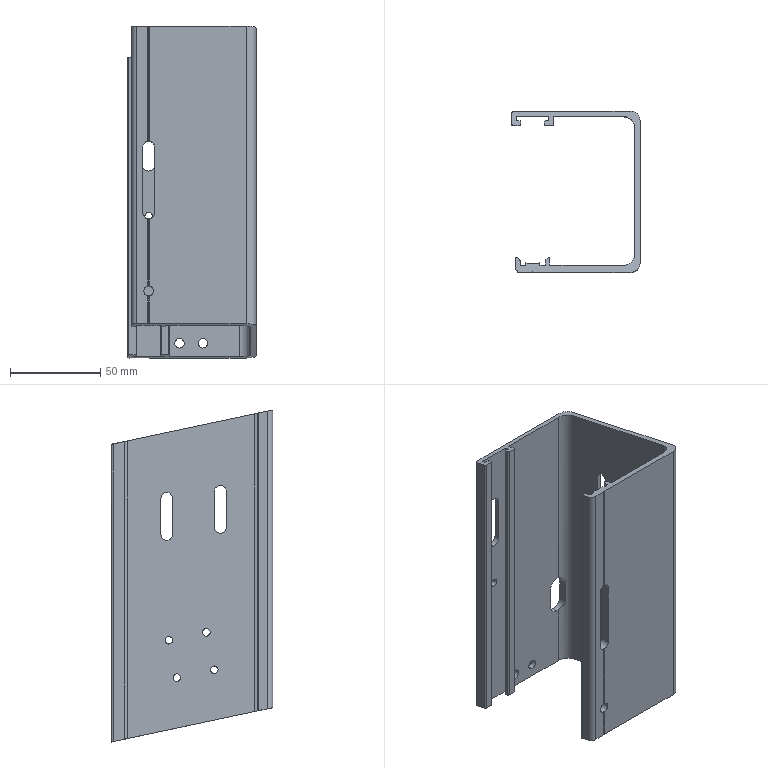Part | STEP file | 31E-01009XJ13 | 1 solid | 106 faces | box 71 x 89.5 x 184.024 mm | volume 127988 mm3 | cylinder 55 | plane 51 | commonest cylinder face diameters 1 x10 4.2 x10 6.5 x10 5.2 x4 8 x4 10 x4